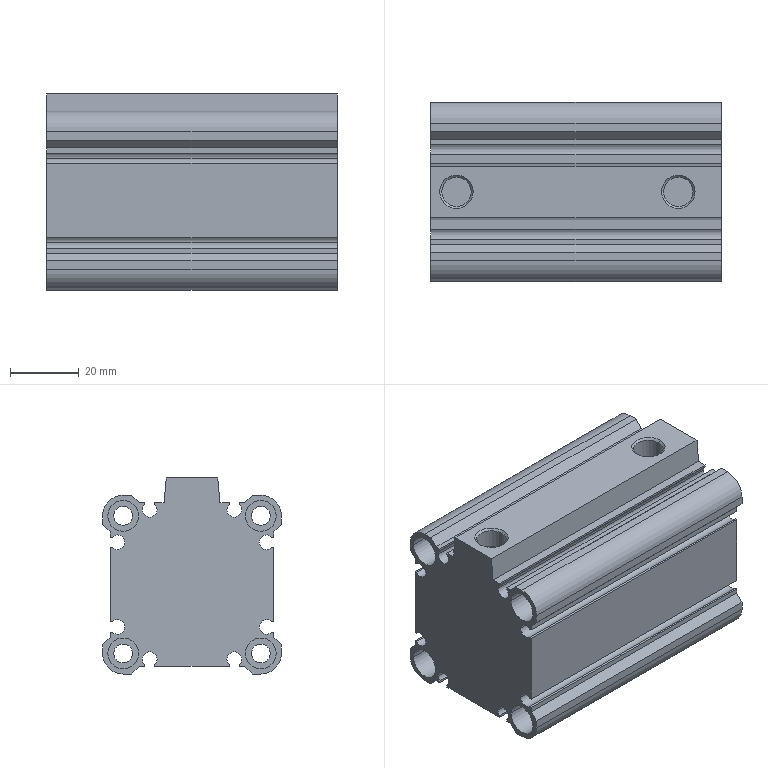Part | STEP file | 25A-CDQ2B40-45DZ-M9BWSDPC-Part-1 | 1 solid | 126 faces | box 84.5 x 52 x 57 mm | volume 122749 mm3 | plane 64 | cylinder 58 | cone 4 | commonest cylinder face diameters 4.26 x18 9 x16 5.5 x8 8.566 x4 12 x4 16 x2